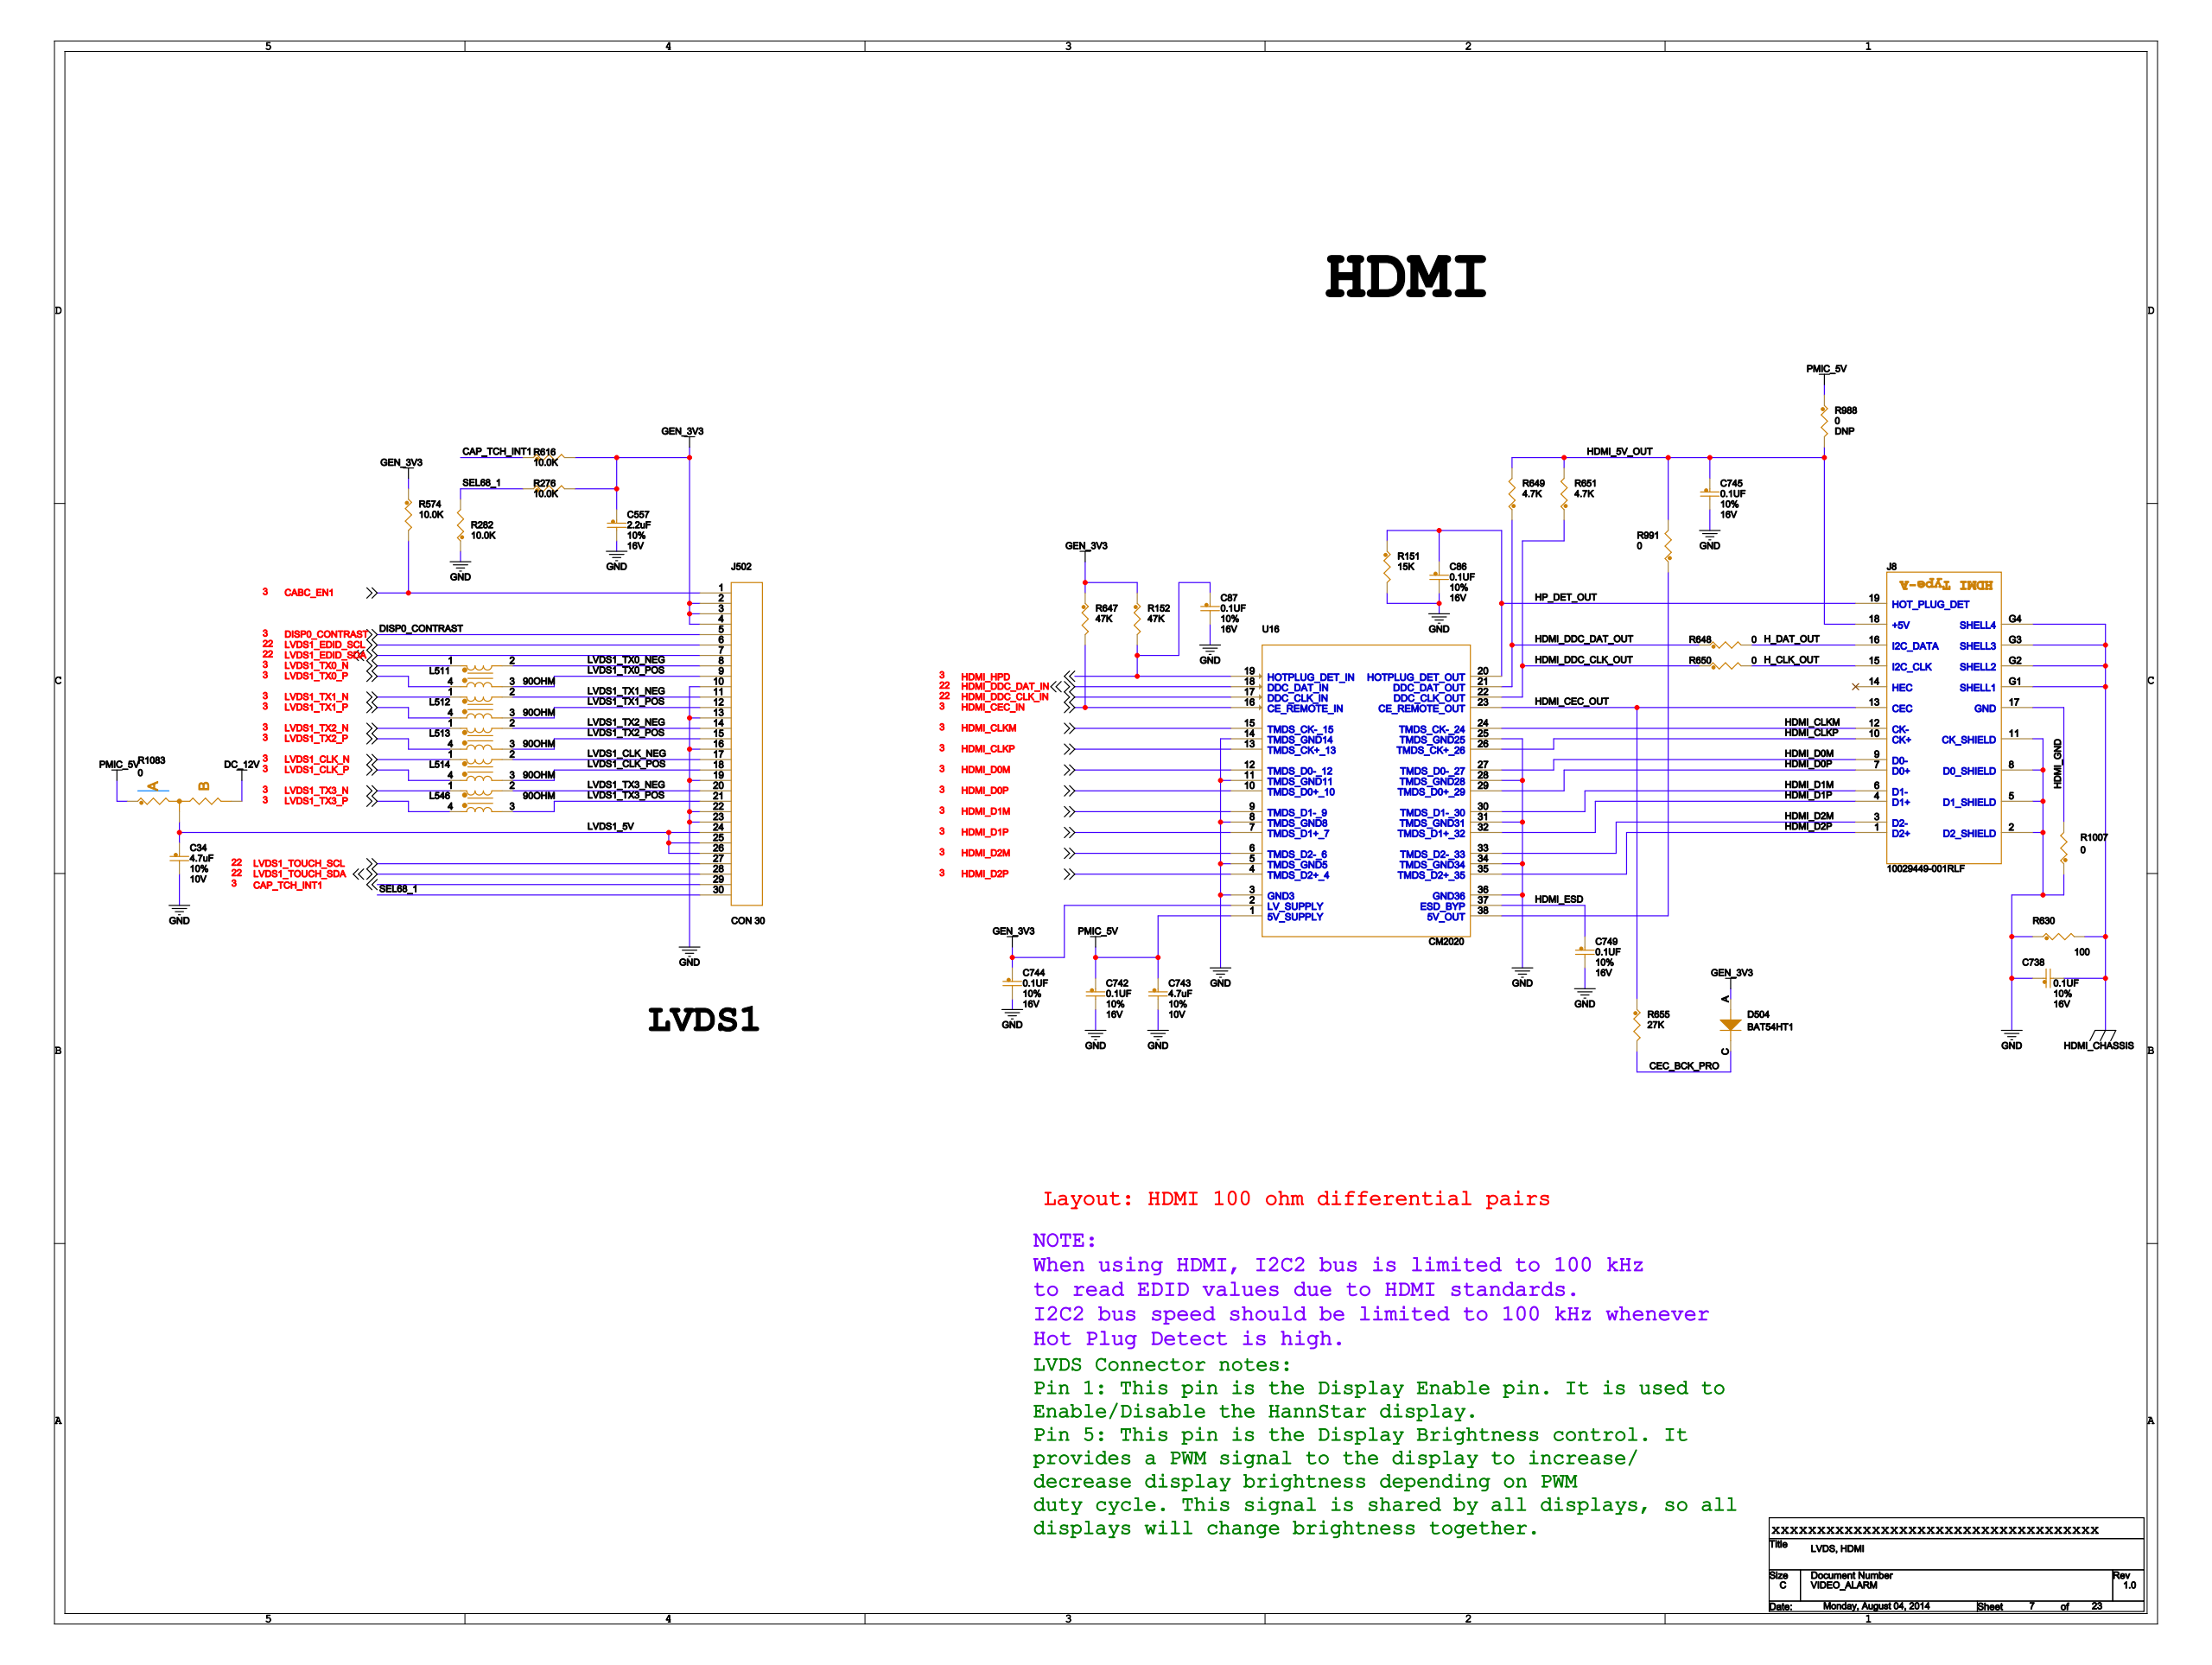Circuit board | Cadence Allegro | 994 parts | 728 nets | one sheet of the schematic
Parts on this sheet (reference | value | footprint):
C34 | 4.7uF | 0603_CC
C86 | 0.1UF | 0603_CC
C87 | 0.1UF | 0603_CC
C557 | 2.2uF | 0603_CC
C738 | 0.1UF | 0603_CC
C742 | 0.1UF | 0603_CC
C743 | 4.7uF | 0603_CC
C744 | 0.1UF | 0603_CC
C745 | 0.1UF | 0603_CC
C749 | 0.1UF | 0603_CC
D504 | BAT54HT1 | SOD323
J8 | 10029449-001RLF | HDMI
J502 | CON 30 | CON_2X15_2_0
L511 | 90OHM | IND4_CHOKE_0805
L512 | 90OHM | IND4_CHOKE_0805
L513 | 90OHM | IND4_CHOKE_0805
L514 | 90OHM | IND4_CHOKE_0805
L546 | 90OHM | IND4_CHOKE_0805
R151 | 15K | 0603_CC
R152 | 47K | 0603_CC
R276 | 10.0K | 0603_CC
R282 | 10.0K | 0603_CC
R574 | 10.0K | 0603_CC
R616 | 10.0K | 0603_CC
R630 | 100 | 0603_CC
R647 | 47K | 0603_CC
R648 | 0 | 0603_CC
R649 | 4.7K | 0603_CC
R650 | 0 | 0603_CC
R651 | 4.7K | 0603_CC
R655 | 27K | 0603_CC
R988 | 0 | 0603_CC
R991 | 0 | 0603_CC
R1007 | 0 | 0603_CC
R1083 | 0 | R0805-X2
U16 | CM2020 | TSSOP38_0P5_4P5X9P8
Nets of these parts (net: part-pin ...):
GND: C34-2 C86-2 C87-2 C557-2 C738-1 C742-2 C743-2 C744-2 C745-2 C749-2 R151-2 R282-1 R630-1 R1007-1 J8-2 J8-5 J8-8 J8-11 J502-10 J502-13 J502-16 J502-19 J502-22 J502-23 U16-3 U16-5 U16-8 U16-11 U16-14 U16-25 U16-28 U16-31 U16-34 U16-36
GEN_3V3: C557-1 C744-1 D504-A R152-1 R276-2 R574-1 R616-2 R647-1 J502-2 J502-3 J502-4 U16-2
PMIC_5V: C742-1 C743-1 R988-1 R1083-1 U16-1
DC_12V: R1083-3
CABC_EN1: R574-2 J502-1
DISP0_CONTRAST: J502-5
LVDS1_EDID_SCL: J502-6
LVDS1_EDID_SDA: J502-7
LVDS1_TX0_POS: L511-3 J502-9
LVDS1_TX0_NEG: L511-2 J502-8
LVDS1_TX1_NEG: L512-2 J502-11
LVDS1_TX1_POS: L512-3 J502-12
LVDS1_TX2_NEG: L513-2 J502-14
LVDS1_TX2_POS: L513-3 J502-15
LVDS1_CLK_NEG: L514-2 J502-17
LVDS1_CLK_POS: L514-3 J502-18
LVDS1_TX3_POS: L546-3 J502-21
LVDS1_TX3_NEG: L546-2 J502-20
LVDS1_5V: C34-1 R1083-2 J502-24 J502-25 J502-26
LVDS1_TOUCH_SCL: J502-27
CAP_TCH_INT1: R616-1 J502-29
LVDS1_TOUCH_SDA: J502-28
SEL68_1: R276-1 R282-2 J502-30
HDMI_CHASSIS: C738-2 R630-2 J8-G1 J8-G2 J8-G3 J8-G4
H_CLK_OUT: R650-2 J8-15
H_DAT_OUT: R648-2 J8-16
HDMI_GND: R1007-2 J8-17
HDMI_5V_OUT: C745-1 R649-2 R651-2 R988-2 R991-2 J8-18
HP_DET_OUT: C86-1 R151-1 J8-19 U16-20
HDMI_D0M: J8-9 U16-12 U16-27
HDMI_CLKP: J8-10 U16-13 U16-26
HDMI_CLKM: J8-12 U16-15 U16-24
HDMI_CEC_OUT: R655-1 J8-13 U16-23
HDMI_D2M: J8-3 U16-6 U16-33
HDMI_D1P: J8-4 U16-7 U16-32
HDMI_D1M: J8-6 U16-9 U16-30
HDMI_D0P: J8-7 U16-10 U16-29
HDMI_D2P: J8-1 U16-4 U16-35
CEC_BCK_PRO: D504-C R655-2
HDMI_CEC_IN: R647-2 U16-16
HDMI_HPD: C87-1 R152-2 U16-19
N19542157: R991-1 U16-38
HDMI_DDC_CLK_OUT: R650-1 R651-1 U16-22
HDMI_DDC_DAT_OUT: R648-1 R649-1 U16-21
HDMI_DDC_CLK_IN: U16-17
HDMI_DDC_DAT_IN: U16-18
HDMI_ESD: C749-1 U16-37
LVDS1_CLK_N: L514-1
LVDS1_CLK_P: L514-4
LVDS1_TX0_N: L511-1
LVDS1_TX0_P: L511-4
LVDS1_TX1_N: L512-1
LVDS1_TX1_P: L512-4
LVDS1_TX2_N: L513-1
LVDS1_TX2_P: L513-4
LVDS1_TX3_N: L546-1
LVDS1_TX3_P: L546-4